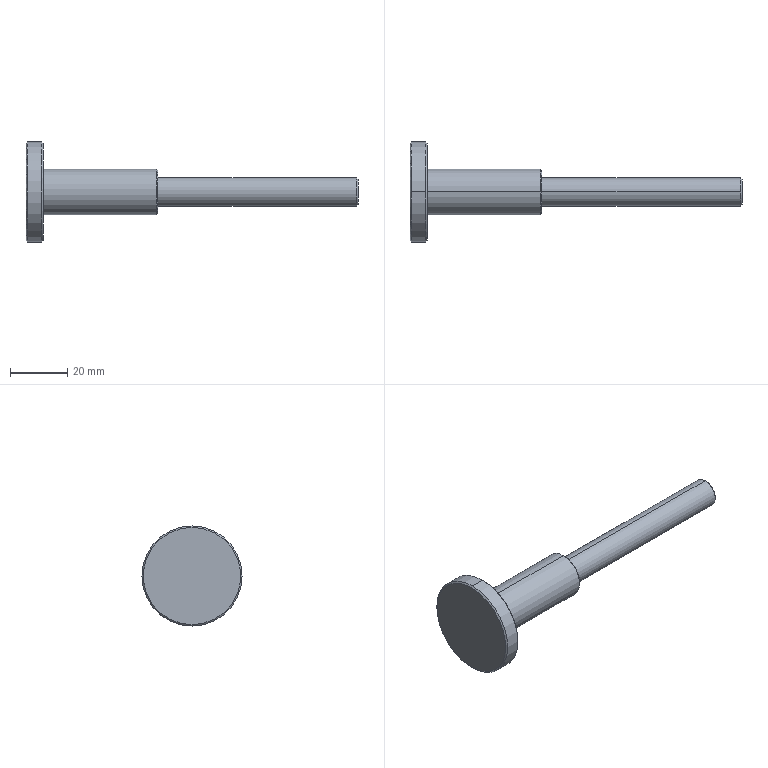Part | SolidWorks | features Chamfer 2, Revolution 1 | 1 solid | 18 faces | box 116 x 35 x 35 mm | volume 19276 mm3 | cone 8 | cylinder 6 | plane 4 | commonest cylinder face diameters 10 x2 16 x2 35 x2
STEP:
#1=CARTESIAN_POINT('',(116.,0.,-4.5));
#2=VERTEX_POINT('',#1);
#3=CARTESIAN_POINT('',(116.,0.,4.5));
#4=VERTEX_POINT('',#3);
#5=CARTESIAN_POINT('',(116.,0.,0.));
#6=DIRECTION('',(1.,0.,0.));
#7=DIRECTION('',(0.,0.,1.));
#8=AXIS2_PLACEMENT_3D('',#5,#6,#7);
#9=CIRCLE('',#8,4.5);
#10=EDGE_CURVE('',#2,#4,#9,.T.);
#11=ORIENTED_EDGE('',*,*,#10,.F.);
#12=CARTESIAN_POINT('',(115.5,0.,-5.));
#13=VERTEX_POINT('',#12);
#14=CARTESIAN_POINT('',(115.5,0.,-5.));
#15=DIRECTION('',(-0.7071,0.,-0.7071));
#16=VECTOR('',#15,1000.);
#17=LINE('',#14,#16);
#18=EDGE_CURVE('',#2,#13,#17,.T.);
#19=ORIENTED_EDGE('',*,*,#18,.T.);
#20=CARTESIAN_POINT('',(115.5,0.,5.));
#21=VERTEX_POINT('',#20);
#22=CARTESIAN_POINT('',(115.5,0.,0.));
#23=DIRECTION('',(-1.,0.,0.));
#24=DIRECTION('',(0.,0.,1.));
#25=AXIS2_PLACEMENT_3D('',#22,#23,#24);
#26=CIRCLE('',#25,5.);
#27=EDGE_CURVE('',#21,#13,#26,.T.);
#28=ORIENTED_EDGE('',*,*,#27,.F.);
#29=CARTESIAN_POINT('',(115.5,0.,5.));
#30=DIRECTION('',(-0.7071,0.,0.7071));
#31=VECTOR('',#30,1000.);
#32=LINE('',#29,#31);
#33=EDGE_CURVE('',#4,#21,#32,.T.);
#34=ORIENTED_EDGE('',*,*,#33,.F.);
#35=EDGE_LOOP('',(#11,#19,#28,#34));
#36=FACE_OUTER_BOUND('',#35,.T.);
#37=CARTESIAN_POINT('',(115.5,0.,0.));
#38=DIRECTION('',(-1.,0.,0.));
#39=DIRECTION('',(0.,0.,1.));
#40=AXIS2_PLACEMENT_3D('',#37,#38,#39);
#41=CONICAL_SURFACE('',#40,5.,0.7854);
#42=ADVANCED_FACE('',(#36),#41,.T.);
#43=CARTESIAN_POINT('',(0.,0.,17.));
#44=VERTEX_POINT('',#43);
#45=CARTESIAN_POINT('',(0.,0.,-17.));
#46=VERTEX_POINT('',#45);
#47=CARTESIAN_POINT('',(0.,0.,0.));
#48=DIRECTION('',(-1.,0.,0.));
#49=DIRECTION('',(0.,0.,-1.));
#50=AXIS2_PLACEMENT_3D('',#47,#48,#49);
#51=CIRCLE('',#50,17.);
#52=EDGE_CURVE('',#44,#46,#51,.T.);
#53=ORIENTED_EDGE('',*,*,#52,.F.);
#54=CARTESIAN_POINT('',(0.5,0.,17.5));
#55=VERTEX_POINT('',#54);
#56=CARTESIAN_POINT('',(0.,0.,17.));
#57=DIRECTION('',(0.7071,0.,0.7071));
#58=VECTOR('',#57,1000.);
#59=LINE('',#56,#58);
#60=EDGE_CURVE('',#44,#55,#59,.T.);
#61=ORIENTED_EDGE('',*,*,#60,.T.);
#62=CARTESIAN_POINT('',(0.5,0.,-17.5));
#63=VERTEX_POINT('',#62);
#64=CARTESIAN_POINT('',(0.5,0.,0.));
#65=DIRECTION('',(1.,0.,0.));
#66=DIRECTION('',(0.,0.,-1.));
#67=AXIS2_PLACEMENT_3D('',#64,#65,#66);
#68=CIRCLE('',#67,17.5);
#69=EDGE_CURVE('',#63,#55,#68,.T.);
#70=ORIENTED_EDGE('',*,*,#69,.F.);
#71=CARTESIAN_POINT('',(0.,0.,-17.));
#72=DIRECTION('',(0.7071,0.,-0.7071));
#73=VECTOR('',#72,1000.);
#74=LINE('',#71,#73);
#75=EDGE_CURVE('',#46,#63,#74,.T.);
#76=ORIENTED_EDGE('',*,*,#75,.F.);
#77=EDGE_LOOP('',(#53,#61,#70,#76));
#78=FACE_OUTER_BOUND('',#77,.T.);
#79=CARTESIAN_POINT('',(0.,0.,0.));
#80=DIRECTION('',(1.,0.,0.));
#81=DIRECTION('',(0.,0.,-1.));
#82=AXIS2_PLACEMENT_3D('',#79,#80,#81);
#83=CONICAL_SURFACE('',#82,17.,0.7854);
#84=ADVANCED_FACE('',(#78),#83,.T.);
#85=CARTESIAN_POINT('',(6.,0.,-17.));
#86=VERTEX_POINT('',#85);
#87=CARTESIAN_POINT('',(6.,0.,17.));
#88=VERTEX_POINT('',#87);
#89=CARTESIAN_POINT('',(6.,0.,0.));
#90=DIRECTION('',(1.,0.,0.));
#91=DIRECTION('',(0.,0.,1.));
#92=AXIS2_PLACEMENT_3D('',#89,#90,#91);
#93=CIRCLE('',#92,17.);
#94=EDGE_CURVE('',#86,#88,#93,.T.);
#95=ORIENTED_EDGE('',*,*,#94,.F.);
#96=CARTESIAN_POINT('',(5.5,0.,-17.5));
#97=VERTEX_POINT('',#96);
#98=CARTESIAN_POINT('',(5.5,0.,-17.5));
#99=DIRECTION('',(-0.7071,0.,-0.7071));
#100=VECTOR('',#99,1000.);
#101=LINE('',#98,#100);
#102=EDGE_CURVE('',#86,#97,#101,.T.);
#103=ORIENTED_EDGE('',*,*,#102,.T.);
#104=CARTESIAN_POINT('',(5.5,0.,17.5));
#105=VERTEX_POINT('',#104);
#106=CARTESIAN_POINT('',(5.5,0.,0.));
#107=DIRECTION('',(-1.,0.,0.));
#108=DIRECTION('',(0.,0.,1.));
#109=AXIS2_PLACEMENT_3D('',#106,#107,#108);
#110=CIRCLE('',#109,17.5);
#111=EDGE_CURVE('',#105,#97,#110,.T.);
#112=ORIENTED_EDGE('',*,*,#111,.F.);
#113=CARTESIAN_POINT('',(5.5,0.,17.5));
#114=DIRECTION('',(-0.7071,0.,0.7071));
#115=VECTOR('',#114,1000.);
#116=LINE('',#113,#115);
#117=EDGE_CURVE('',#88,#105,#116,.T.);
#118=ORIENTED_EDGE('',*,*,#117,.F.);
#119=EDGE_LOOP('',(#95,#103,#112,#118));
#120=FACE_OUTER_BOUND('',#119,.T.);
#121=CARTESIAN_POINT('',(5.5,0.,0.));
#122=DIRECTION('',(-1.,0.,0.));
#123=DIRECTION('',(0.,0.,1.));
#124=AXIS2_PLACEMENT_3D('',#121,#122,#123);
#125=CONICAL_SURFACE('',#124,17.5,0.7854);
#126=ADVANCED_FACE('',(#120),#125,.T.);
#127=CARTESIAN_POINT('',(46.,0.,-7.5));
#128=VERTEX_POINT('',#127);
#129=CARTESIAN_POINT('',(46.,0.,7.5));
#130=VERTEX_POINT('',#129);
#131=CARTESIAN_POINT('',(46.,0.,0.));
#132=DIRECTION('',(1.,0.,0.));
#133=DIRECTION('',(0.,0.,1.));
#134=AXIS2_PLACEMENT_3D('',#131,#132,#133);
#135=CIRCLE('',#134,7.5);
#136=EDGE_CURVE('',#128,#130,#135,.T.);
#137=ORIENTED_EDGE('',*,*,#136,.F.);
#138=CARTESIAN_POINT('',(45.5,0.,-8.));
#139=VERTEX_POINT('',#138);
#140=CARTESIAN_POINT('',(45.5,0.,-8.));
#141=DIRECTION('',(-0.7071,0.,-0.7071));
#142=VECTOR('',#141,1000.);
#143=LINE('',#140,#142);
#144=EDGE_CURVE('',#128,#139,#143,.T.);
#145=ORIENTED_EDGE('',*,*,#144,.T.);
#146=CARTESIAN_POINT('',(45.5,0.,8.));
#147=VERTEX_POINT('',#146);
#148=CARTESIAN_POINT('',(45.5,0.,0.));
#149=DIRECTION('',(-1.,0.,0.));
#150=DIRECTION('',(0.,0.,1.));
#151=AXIS2_PLACEMENT_3D('',#148,#149,#150);
#152=CIRCLE('',#151,8.);
#153=EDGE_CURVE('',#147,#139,#152,.T.);
#154=ORIENTED_EDGE('',*,*,#153,.F.);
#155=CARTESIAN_POINT('',(45.5,0.,8.));
#156=DIRECTION('',(-0.7071,0.,0.7071));
#157=VECTOR('',#156,1000.);
#158=LINE('',#155,#157);
#159=EDGE_CURVE('',#130,#147,#158,.T.);
#160=ORIENTED_EDGE('',*,*,#159,.F.);
#161=EDGE_LOOP('',(#137,#145,#154,#160));
#162=FACE_OUTER_BOUND('',#161,.T.);
#163=CARTESIAN_POINT('',(45.5,0.,0.));
#164=DIRECTION('',(-1.,0.,0.));
#165=DIRECTION('',(0.,0.,1.));
#166=AXIS2_PLACEMENT_3D('',#163,#164,#165);
#167=CONICAL_SURFACE('',#166,8.,0.7854);
#168=ADVANCED_FACE('',(#162),#167,.T.);
#169=ORIENTED_EDGE('',*,*,#27,.T.);
#170=CARTESIAN_POINT('',(46.,0.,-5.));
#171=VERTEX_POINT('',#170);
#172=CARTESIAN_POINT('',(0.,0.,-5.));
#173=DIRECTION('',(-1.,0.,0.));
#174=VECTOR('',#173,1000.);
#175=LINE('',#172,#174);
#176=EDGE_CURVE('',#13,#171,#175,.T.);
#177=ORIENTED_EDGE('',*,*,#176,.T.);
#178=CARTESIAN_POINT('',(46.,0.,5.));
#179=VERTEX_POINT('',#178);
#180=CARTESIAN_POINT('',(46.,0.,0.));
#181=DIRECTION('',(-1.,0.,0.));
#182=DIRECTION('',(0.,0.,1.));
#183=AXIS2_PLACEMENT_3D('',#180,#181,#182);
#184=CIRCLE('',#183,5.);
#185=EDGE_CURVE('',#179,#171,#184,.T.);
#186=ORIENTED_EDGE('',*,*,#185,.F.);
#187=CARTESIAN_POINT('',(0.,0.,5.));
#188=DIRECTION('',(-1.,0.,0.));
#189=VECTOR('',#188,1000.);
#190=LINE('',#187,#189);
#191=EDGE_CURVE('',#21,#179,#190,.T.);
#192=ORIENTED_EDGE('',*,*,#191,.F.);
#193=EDGE_LOOP('',(#169,#177,#186,#192));
#194=FACE_OUTER_BOUND('',#193,.T.);
#195=CARTESIAN_POINT('',(0.,0.,0.));
#196=DIRECTION('',(-1.,0.,0.));
#197=DIRECTION('',(0.,0.,1.));
#198=AXIS2_PLACEMENT_3D('',#195,#196,#197);
#199=CYLINDRICAL_SURFACE('',#198,5.);
#200=ADVANCED_FACE('',(#194),#199,.T.);
#201=ORIENTED_EDGE('',*,*,#153,.T.);
#202=CARTESIAN_POINT('',(6.,0.,-8.));
#203=VERTEX_POINT('',#202);
#204=CARTESIAN_POINT('',(0.,0.,-8.));
#205=DIRECTION('',(-1.,0.,0.));
#206=VECTOR('',#205,1000.);
#207=LINE('',#204,#206);
#208=EDGE_CURVE('',#139,#203,#207,.T.);
#209=ORIENTED_EDGE('',*,*,#208,.T.);
#210=CARTESIAN_POINT('',(6.,0.,8.));
#211=VERTEX_POINT('',#210);
#212=CARTESIAN_POINT('',(6.,0.,0.));
#213=DIRECTION('',(-1.,0.,0.));
#214=DIRECTION('',(0.,0.,1.));
#215=AXIS2_PLACEMENT_3D('',#212,#213,#214);
#216=CIRCLE('',#215,8.);
#217=EDGE_CURVE('',#211,#203,#216,.T.);
#218=ORIENTED_EDGE('',*,*,#217,.F.);
#219=CARTESIAN_POINT('',(0.,0.,8.));
#220=DIRECTION('',(-1.,0.,0.));
#221=VECTOR('',#220,1000.);
#222=LINE('',#219,#221);
#223=EDGE_CURVE('',#147,#211,#222,.T.);
#224=ORIENTED_EDGE('',*,*,#223,.F.);
#225=EDGE_LOOP('',(#201,#209,#218,#224));
#226=FACE_OUTER_BOUND('',#225,.T.);
#227=CARTESIAN_POINT('',(0.,0.,0.));
#228=DIRECTION('',(-1.,0.,0.));
#229=DIRECTION('',(0.,0.,1.));
#230=AXIS2_PLACEMENT_3D('',#227,#228,#229);
#231=CYLINDRICAL_SURFACE('',#230,8.);
#232=ADVANCED_FACE('',(#226),#231,.T.);
#233=ORIENTED_EDGE('',*,*,#111,.T.);
#234=CARTESIAN_POINT('',(0.,0.,-17.5));
#235=DIRECTION('',(-1.,0.,0.));
#236=VECTOR('',#235,1000.);
#237=LINE('',#234,#236);
#238=EDGE_CURVE('',#97,#63,#237,.T.);
#239=ORIENTED_EDGE('',*,*,#238,.T.);
#240=ORIENTED_EDGE('',*,*,#69,.T.);
#241=CARTESIAN_POINT('',(0.,0.,17.5));
#242=DIRECTION('',(-1.,0.,0.));
#243=VECTOR('',#242,1000.);
#244=LINE('',#241,#243);
#245=EDGE_CURVE('',#105,#55,#244,.T.);
#246=ORIENTED_EDGE('',*,*,#245,.F.);
#247=EDGE_LOOP('',(#233,#239,#240,#246));
#248=FACE_OUTER_BOUND('',#247,.T.);
#249=CARTESIAN_POINT('',(0.,0.,0.));
#250=DIRECTION('',(-1.,0.,0.));
#251=DIRECTION('',(0.,0.,1.));
#252=AXIS2_PLACEMENT_3D('',#249,#250,#251);
#253=CYLINDRICAL_SURFACE('',#252,17.5);
#254=ADVANCED_FACE('',(#248),#253,.T.);
#255=CARTESIAN_POINT('',(0.,0.,0.));
#256=DIRECTION('',(-1.,0.,0.));
#257=DIRECTION('',(0.,0.,-1.));
#258=AXIS2_PLACEMENT_3D('',#255,#256,#257);
#259=CIRCLE('',#258,17.);
#260=EDGE_CURVE('',#46,#44,#259,.T.);
#261=ORIENTED_EDGE('',*,*,#260,.T.);
#262=ORIENTED_EDGE('',*,*,#52,.T.);
#263=EDGE_LOOP('',(#261,#262));
#264=FACE_OUTER_BOUND('',#263,.T.);
#265=CARTESIAN_POINT('',(0.,0.,0.));
#266=DIRECTION('',(1.,0.,0.));
#267=DIRECTION('',(0.,0.,-1.));
#268=AXIS2_PLACEMENT_3D('',#265,#266,#267);
#269=PLANE('',#268);
#270=ADVANCED_FACE('',(#264),#269,.F.);
#271=ORIENTED_EDGE('',*,*,#238,.F.);
#272=CARTESIAN_POINT('',(5.5,0.,0.));
#273=DIRECTION('',(-1.,0.,0.));
#274=DIRECTION('',(0.,0.,1.));
#275=AXIS2_PLACEMENT_3D('',#272,#273,#274);
#276=CIRCLE('',#275,17.5);
#277=EDGE_CURVE('',#97,#105,#276,.T.);
#278=ORIENTED_EDGE('',*,*,#277,.T.);
#279=ORIENTED_EDGE('',*,*,#245,.T.);
#280=CARTESIAN_POINT('',(0.5,0.,0.));
#281=DIRECTION('',(1.,0.,0.));
#282=DIRECTION('',(0.,0.,-1.));
#283=AXIS2_PLACEMENT_3D('',#280,#281,#282);
#284=CIRCLE('',#283,17.5);
#285=EDGE_CURVE('',#55,#63,#284,.T.);
#286=ORIENTED_EDGE('',*,*,#285,.T.);
#287=EDGE_LOOP('',(#271,#278,#279,#286));
#288=FACE_OUTER_BOUND('',#287,.T.);
#289=CARTESIAN_POINT('',(0.,0.,0.));
#290=DIRECTION('',(-1.,0.,0.));
#291=DIRECTION('',(0.,0.,1.));
#292=AXIS2_PLACEMENT_3D('',#289,#290,#291);
#293=CYLINDRICAL_SURFACE('',#292,17.5);
#294=ADVANCED_FACE('',(#288),#293,.T.);
#295=CARTESIAN_POINT('',(6.,0.,0.));
#296=DIRECTION('',(1.,0.,0.));
#297=DIRECTION('',(0.,0.,1.));
#298=AXIS2_PLACEMENT_3D('',#295,#296,#297);
#299=CIRCLE('',#298,17.);
#300=EDGE_CURVE('',#88,#86,#299,.T.);
#301=ORIENTED_EDGE('',*,*,#300,.T.);
#302=ORIENTED_EDGE('',*,*,#94,.T.);
#303=EDGE_LOOP('',(#301,#302));
#304=FACE_OUTER_BOUND('',#303,.T.);
#305=ORIENTED_EDGE('',*,*,#217,.T.);
#306=CARTESIAN_POINT('',(6.,0.,0.));
#307=DIRECTION('',(-1.,0.,0.));
#308=DIRECTION('',(0.,0.,1.));
#309=AXIS2_PLACEMENT_3D('',#306,#307,#308);
#310=CIRCLE('',#309,8.);
#311=EDGE_CURVE('',#203,#211,#310,.T.);
#312=ORIENTED_EDGE('',*,*,#311,.T.);
#313=EDGE_LOOP('',(#305,#312));
#314=FACE_BOUND('',#313,.T.);
#315=CARTESIAN_POINT('',(6.,17.5,0.));
#316=DIRECTION('',(-1.,0.,0.));
#317=DIRECTION('',(0.,0.,1.));
#318=AXIS2_PLACEMENT_3D('',#315,#316,#317);
#319=PLANE('',#318);
#320=ADVANCED_FACE('',(#304,#314),#319,.F.);
#321=ORIENTED_EDGE('',*,*,#208,.F.);
#322=CARTESIAN_POINT('',(45.5,0.,0.));
#323=DIRECTION('',(-1.,0.,0.));
#324=DIRECTION('',(0.,0.,1.));
#325=AXIS2_PLACEMENT_3D('',#322,#323,#324);
#326=CIRCLE('',#325,8.);
#327=EDGE_CURVE('',#139,#147,#326,.T.);
#328=ORIENTED_EDGE('',*,*,#327,.T.);
#329=ORIENTED_EDGE('',*,*,#223,.T.);
#330=ORIENTED_EDGE('',*,*,#311,.F.);
#331=EDGE_LOOP('',(#321,#328,#329,#330));
#332=FACE_OUTER_BOUND('',#331,.T.);
#333=CARTESIAN_POINT('',(0.,0.,0.));
#334=DIRECTION('',(-1.,0.,0.));
#335=DIRECTION('',(0.,0.,1.));
#336=AXIS2_PLACEMENT_3D('',#333,#334,#335);
#337=CYLINDRICAL_SURFACE('',#336,8.);
#338=ADVANCED_FACE('',(#332),#337,.T.);
#339=CARTESIAN_POINT('',(46.,0.,0.));
#340=DIRECTION('',(1.,0.,0.));
#341=DIRECTION('',(0.,0.,1.));
#342=AXIS2_PLACEMENT_3D('',#339,#340,#341);
#343=CIRCLE('',#342,7.5);
#344=EDGE_CURVE('',#130,#128,#343,.T.);
#345=ORIENTED_EDGE('',*,*,#344,.T.);
#346=ORIENTED_EDGE('',*,*,#136,.T.);
#347=EDGE_LOOP('',(#345,#346));
#348=FACE_OUTER_BOUND('',#347,.T.);
#349=ORIENTED_EDGE('',*,*,#185,.T.);
#350=CARTESIAN_POINT('',(46.,0.,0.));
#351=DIRECTION('',(-1.,0.,0.));
#352=DIRECTION('',(0.,0.,1.));
#353=AXIS2_PLACEMENT_3D('',#350,#351,#352);
#354=CIRCLE('',#353,5.);
#355=EDGE_CURVE('',#171,#179,#354,.T.);
#356=ORIENTED_EDGE('',*,*,#355,.T.);
#357=EDGE_LOOP('',(#349,#356));
#358=FACE_BOUND('',#357,.T.);
#359=CARTESIAN_POINT('',(46.,8.,0.));
#360=DIRECTION('',(-1.,0.,0.));
#361=DIRECTION('',(0.,0.,1.));
#362=AXIS2_PLACEMENT_3D('',#359,#360,#361);
#363=PLANE('',#362);
#364=ADVANCED_FACE('',(#348,#358),#363,.F.);
#365=ORIENTED_EDGE('',*,*,#176,.F.);
#366=CARTESIAN_POINT('',(115.5,0.,0.));
#367=DIRECTION('',(-1.,0.,0.));
#368=DIRECTION('',(0.,0.,1.));
#369=AXIS2_PLACEMENT_3D('',#366,#367,#368);
#370=CIRCLE('',#369,5.);
#371=EDGE_CURVE('',#13,#21,#370,.T.);
#372=ORIENTED_EDGE('',*,*,#371,.T.);
#373=ORIENTED_EDGE('',*,*,#191,.T.);
#374=ORIENTED_EDGE('',*,*,#355,.F.);
#375=EDGE_LOOP('',(#365,#372,#373,#374));
#376=FACE_OUTER_BOUND('',#375,.T.);
#377=CARTESIAN_POINT('',(0.,0.,0.));
#378=DIRECTION('',(-1.,0.,0.));
#379=DIRECTION('',(0.,0.,1.));
#380=AXIS2_PLACEMENT_3D('',#377,#378,#379);
#381=CYLINDRICAL_SURFACE('',#380,5.);
#382=ADVANCED_FACE('',(#376),#381,.T.);
#383=CARTESIAN_POINT('',(116.,0.,0.));
#384=DIRECTION('',(1.,0.,0.));
#385=DIRECTION('',(0.,0.,1.));
#386=AXIS2_PLACEMENT_3D('',#383,#384,#385);
#387=CIRCLE('',#386,4.5);
#388=EDGE_CURVE('',#4,#2,#387,.T.);
#389=ORIENTED_EDGE('',*,*,#388,.T.);
#390=ORIENTED_EDGE('',*,*,#10,.T.);
#391=EDGE_LOOP('',(#389,#390));
#392=FACE_OUTER_BOUND('',#391,.T.);
#393=CARTESIAN_POINT('',(116.,5.,0.));
#394=DIRECTION('',(-1.,0.,0.));
#395=DIRECTION('',(0.,0.,1.));
#396=AXIS2_PLACEMENT_3D('',#393,#394,#395);
#397=PLANE('',#396);
#398=ADVANCED_FACE('',(#392),#397,.F.);
#399=ORIENTED_EDGE('',*,*,#144,.F.);
#400=ORIENTED_EDGE('',*,*,#344,.F.);
#401=ORIENTED_EDGE('',*,*,#159,.T.);
#402=ORIENTED_EDGE('',*,*,#327,.F.);
#403=EDGE_LOOP('',(#399,#400,#401,#402));
#404=FACE_OUTER_BOUND('',#403,.T.);
#405=CARTESIAN_POINT('',(45.5,0.,0.));
#406=DIRECTION('',(-1.,0.,0.));
#407=DIRECTION('',(0.,0.,1.));
#408=AXIS2_PLACEMENT_3D('',#405,#406,#407);
#409=CONICAL_SURFACE('',#408,8.,0.7854);
#410=ADVANCED_FACE('',(#404),#409,.T.);
#411=ORIENTED_EDGE('',*,*,#102,.F.);
#412=ORIENTED_EDGE('',*,*,#300,.F.);
#413=ORIENTED_EDGE('',*,*,#117,.T.);
#414=ORIENTED_EDGE('',*,*,#277,.F.);
#415=EDGE_LOOP('',(#411,#412,#413,#414));
#416=FACE_OUTER_BOUND('',#415,.T.);
#417=CARTESIAN_POINT('',(5.5,0.,0.));
#418=DIRECTION('',(-1.,0.,0.));
#419=DIRECTION('',(0.,0.,1.));
#420=AXIS2_PLACEMENT_3D('',#417,#418,#419);
#421=CONICAL_SURFACE('',#420,17.5,0.7854);
#422=ADVANCED_FACE('',(#416),#421,.T.);
#423=ORIENTED_EDGE('',*,*,#60,.F.);
#424=ORIENTED_EDGE('',*,*,#260,.F.);
#425=ORIENTED_EDGE('',*,*,#75,.T.);
#426=ORIENTED_EDGE('',*,*,#285,.F.);
#427=EDGE_LOOP('',(#423,#424,#425,#426));
#428=FACE_OUTER_BOUND('',#427,.T.);
#429=CARTESIAN_POINT('',(0.,0.,0.));
#430=DIRECTION('',(1.,0.,0.));
#431=DIRECTION('',(0.,0.,-1.));
#432=AXIS2_PLACEMENT_3D('',#429,#430,#431);
#433=CONICAL_SURFACE('',#432,17.,0.7854);
#434=ADVANCED_FACE('',(#428),#433,.T.);
#435=ORIENTED_EDGE('',*,*,#18,.F.);
#436=ORIENTED_EDGE('',*,*,#388,.F.);
#437=ORIENTED_EDGE('',*,*,#33,.T.);
#438=ORIENTED_EDGE('',*,*,#371,.F.);
#439=EDGE_LOOP('',(#435,#436,#437,#438));
#440=FACE_OUTER_BOUND('',#439,.T.);
#441=CARTESIAN_POINT('',(115.5,0.,0.));
#442=DIRECTION('',(-1.,0.,0.));
#443=DIRECTION('',(0.,0.,1.));
#444=AXIS2_PLACEMENT_3D('',#441,#442,#443);
#445=CONICAL_SURFACE('',#444,5.,0.7854);
#446=ADVANCED_FACE('',(#440),#445,.T.);
#447=CLOSED_SHELL('',(#42,#84,#126,#168,#200,#232,#254,#270,#294,#320,#338,#364,#382,#398,#410,#422,#434,#446));
#448=MANIFOLD_SOLID_BREP('',#447);
#449=CARTESIAN_POINT('',(0.,0.,0.));
#450=DIRECTION('',(0.,0.,1.));
#451=DIRECTION('',(1.,0.,0.));
#452=AXIS2_PLACEMENT_3D('',#449,#450,#451);
#453=(LENGTH_UNIT()NAMED_UNIT(*)SI_UNIT(.MILLI.,.METRE.));
#454=UNCERTAINTY_MEASURE_WITH_UNIT(LENGTH_MEASURE(0.00001),#453,'','');
#455=(NAMED_UNIT(*)PLANE_ANGLE_UNIT()SI_UNIT($,.RADIAN.));
#456=(NAMED_UNIT(*)SI_UNIT($,.STERADIAN.)SOLID_ANGLE_UNIT());
#457=(GEOMETRIC_REPRESENTATION_CONTEXT(3)GLOBAL_UNCERTAINTY_ASSIGNED_CONTEXT((#454))GLOBAL_UNIT_ASSIGNED_CONTEXT((#453,#455,#456))REPRESENTATION_CONTEXT('',''));
#458=ADVANCED_BREP_SHAPE_REPRESENTATION('',(#448,#452),#457);